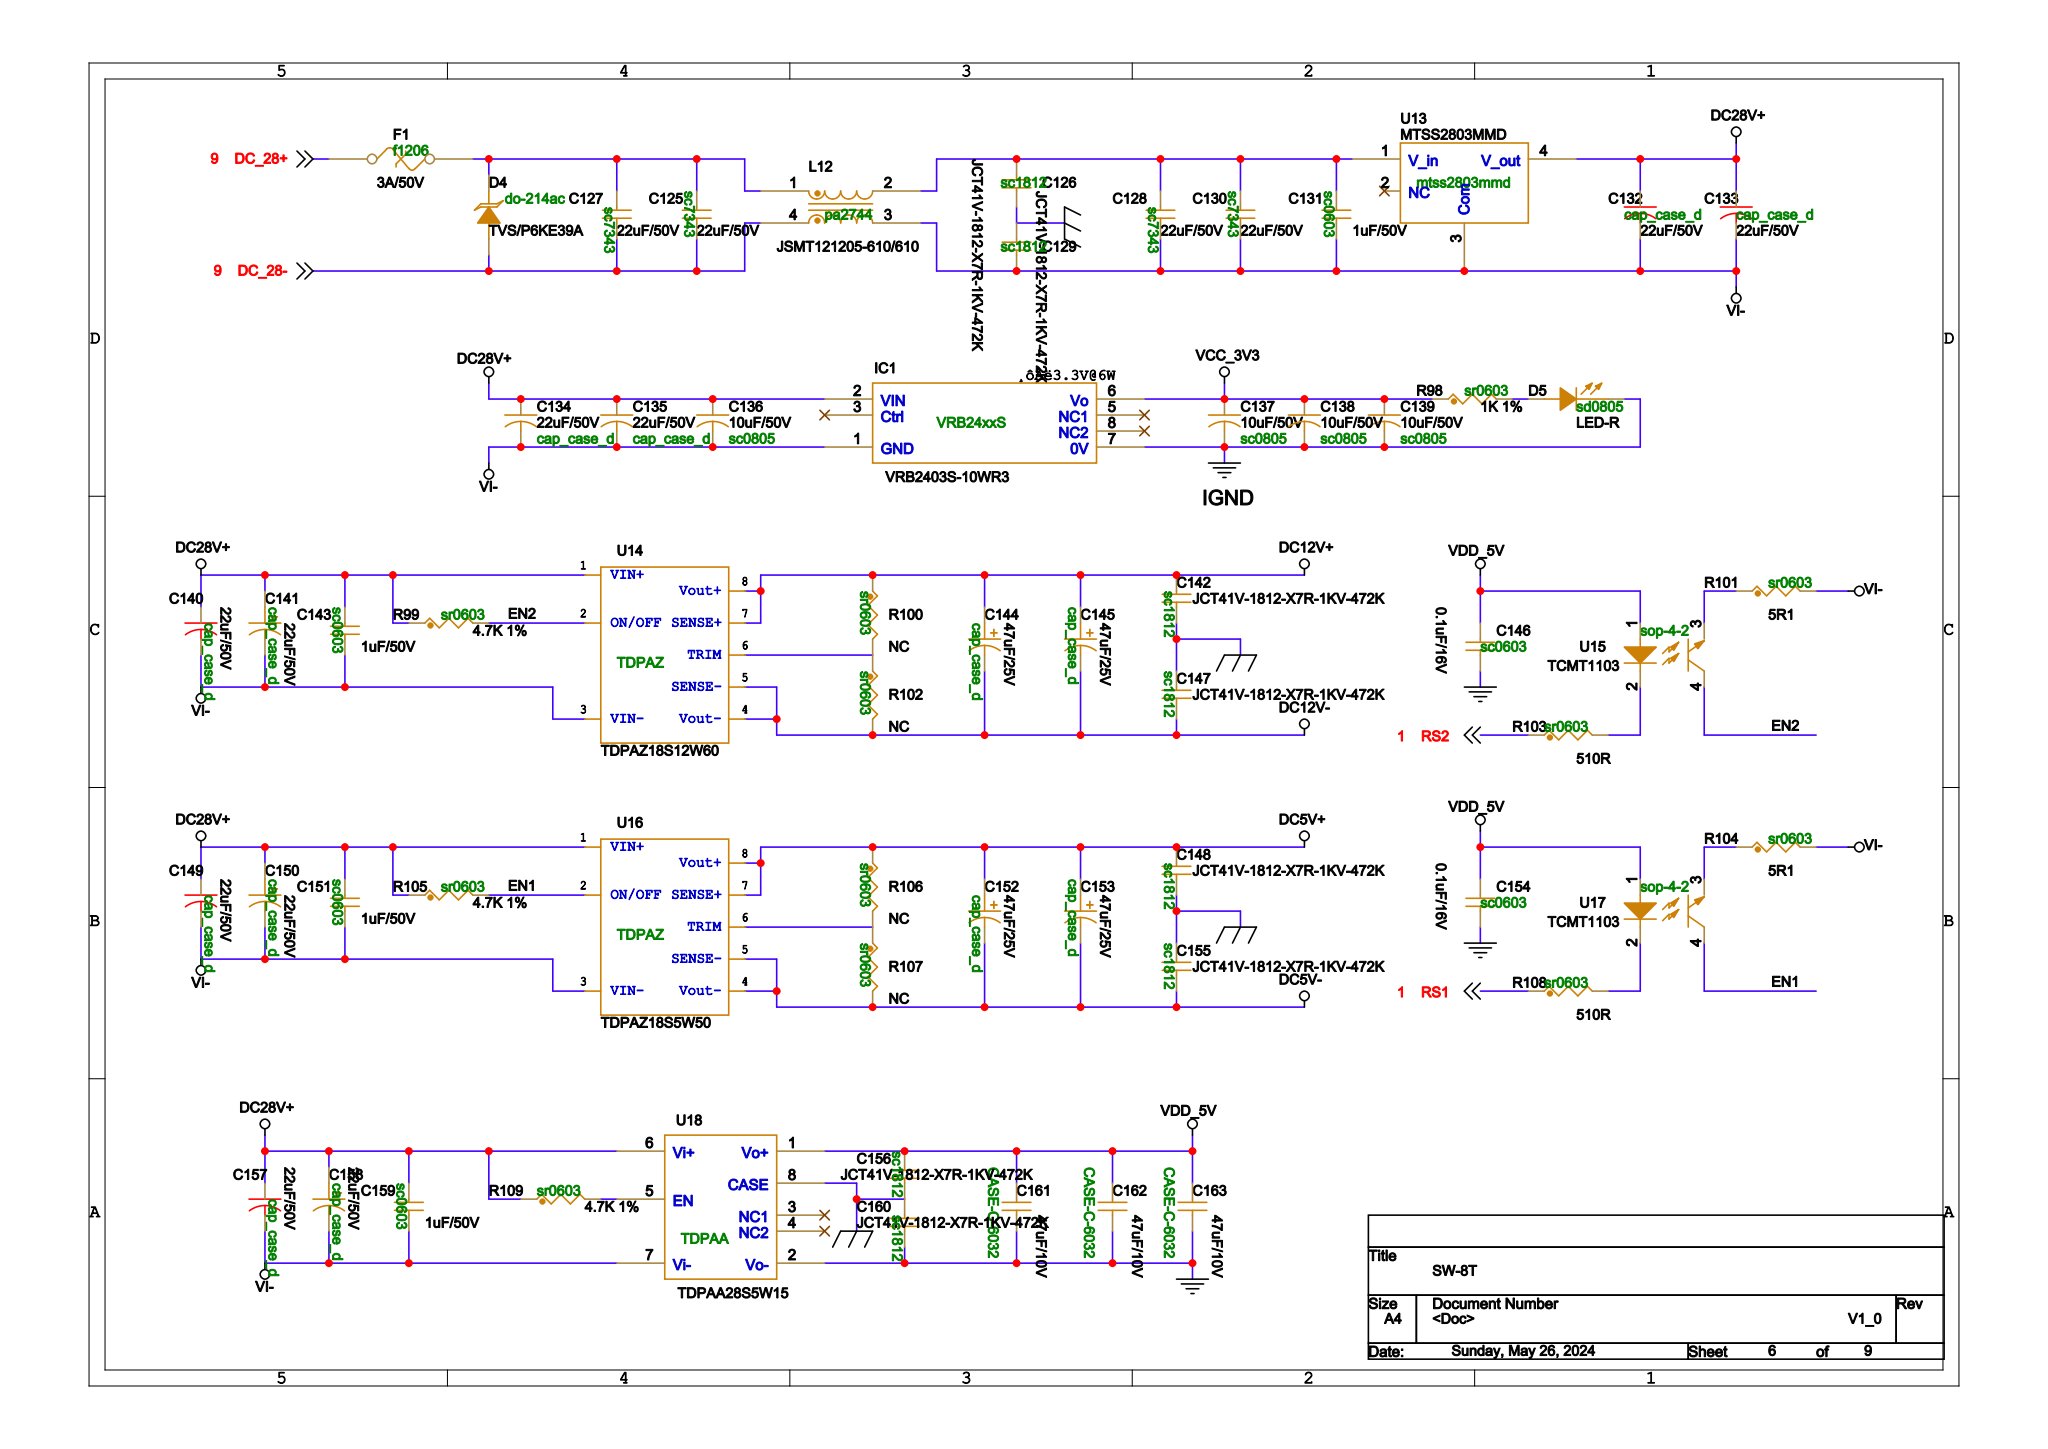Circuit board | Cadence Allegro | 399 parts | 387 nets | one sheet of the schematic
Parts on this sheet (reference | value | footprint):
C125 | 22uF/50V | SC7343
C126 | JCT41V-1812-X7R-1KV-472K | SC1812
C127 | 22uF/50V | SC7343
C128 | 22uF/50V | SC7343
C129 | JCT41V-1812-X7R-1KV-472K | SC1812
C130 | 22uF/50V | SC7343
C131 | 1uF/50V | SC0603
C132 | 22uF/50V | CAP_CASE_D
C133 | 22uF/50V | CAP_CASE_D
C134 | 22uF/50V | CAP_CASE_D
C135 | 22uF/50V | CAP_CASE_D
C136 | 10uF/50V | SC0805
C137 | 10uF/50V | SC0805
C138 | 10uF/50V | SC0805
C139 | 10uF/50V | SC0805
C140 | 22uF/50V | CAP_CASE_D
C142 | JCT41V-1812-X7R-1KV-472K | SC1812
C143 | 1uF/50V | SC0603
C146 | 0.1uF/16V | SC0603
C147 | JCT41V-1812-X7R-1KV-472K | SC1812
C148 | JCT41V-1812-X7R-1KV-472K | SC1812
C149 | 22uF/50V | CAP_CASE_D
C151 | 1uF/50V | SC0603
C154 | 0.1uF/16V | SC0603
C155 | JCT41V-1812-X7R-1KV-472K | SC1812
C156 | JCT41V-1812-X7R-1KV-472K | SC1812
C157 | 22uF/50V | CAP_CASE_D
C159 | 1uF/50V | SC0603
C160 | JCT41V-1812-X7R-1KV-472K | SC1812
D4 | TVS/P6KE39A | DO-214AC
D5 | LED-R | SD0805
F1 | 3A/50V | F1206
IC1 | VRB2403S-10WR3 | VRB24XXS
L12 | JSMT121205-610/610 | PA2744
R98 | 1K 1% | SR0603
R99 | 4.7K 1% | SR0603
R100 | NC | SR0603
R101 | 5R1 | SR0603
R102 | NC | SR0603
R103 | 510R | SR0603
R104 | 5R1 | SR0603
R105 | 4.7K 1% | SR0603
R106 | NC | SR0603
R107 | NC | SR0603
R108 | 510R | SR0603
R109 | 4.7K 1% | SR0603
U13 | MTSS2803MMD | MTSS2803MMD
U14 | TDPAZ18S12W60 | TDPAZ
U15 | TCMT1103 | SOP-4-2
U16 | TDPAZ18S5W50 | TDPAZ
U17 | TCMT1103 | SOP-4-2
U18 | TDPAA28S5W15 | TDPAA
Nets of these parts (net: part-pin ...):
GND: C146-2 C154-2 C160-2 U18-2
VCC_3V3: C137-1 C138-1 C139-1 IC1-6 R98-1
AGND: C137-2 C138-2 C139-2 D5-2 IC1-7
N17728197: C125-1 C127-1 D4-1 F1-2 L12-1
DC_28-: C125-2 C127-2 D4-2 L12-4
N17728207: C126-2 C128-1 C130-1 C131-1 L12-2 U13-1
VI-: C128-2 C129-2 C130-2 C131-2 C132-2 C133-2 C134-2 C135-2 C136-2 C140-2 C143-2 C149-2 C151-2 C157-2 C159-2 IC1-1 L12-3 R101-2 R104-2 U13-3 U14-3 U16-3 U18-7
GND_EARTH: C126-1 C129-1 C142-2 C147-1 C148-2 C155-1 C156-2 C160-1 U18-8
DC12V+: C142-1 R100-1 U14-7 U14-8
DC12V-: C147-2 R102-2 U14-4 U14-5
DC5V+: C148-1 R106-1 U16-7 U16-8
DC5V-: C155-2 R107-2 U16-4 U16-5
VDD_5V: C146-1 C154-1 C156-1 U15-1 U17-1 U18-1
DC28V+: C132-1 C133-1 C134-1 C135-1 C136-1 C140-1 C143-1 C149-1 C151-1 C157-1 C159-1 IC1-2 R99-1 R105-1 R109-1 U13-4 U14-1 U16-1 U18-6
N17848168: D5-1 R98-2
DC_28+: F1-1
N17846513: R100-2 R102-1 U14-6
N17730854: R106-2 R107-1 U16-6
N17849995: R101-1 U15-3
N17736372: R104-1 U17-3
RS2: R103-1
N17849955: R103-2 U15-2
RS1: R108-1
N17736334: R108-2 U17-2
EN1: R105-2 U16-2 U17-4
N17733703: R109-2 U18-5
EN2: R99-2 U14-2 U15-4